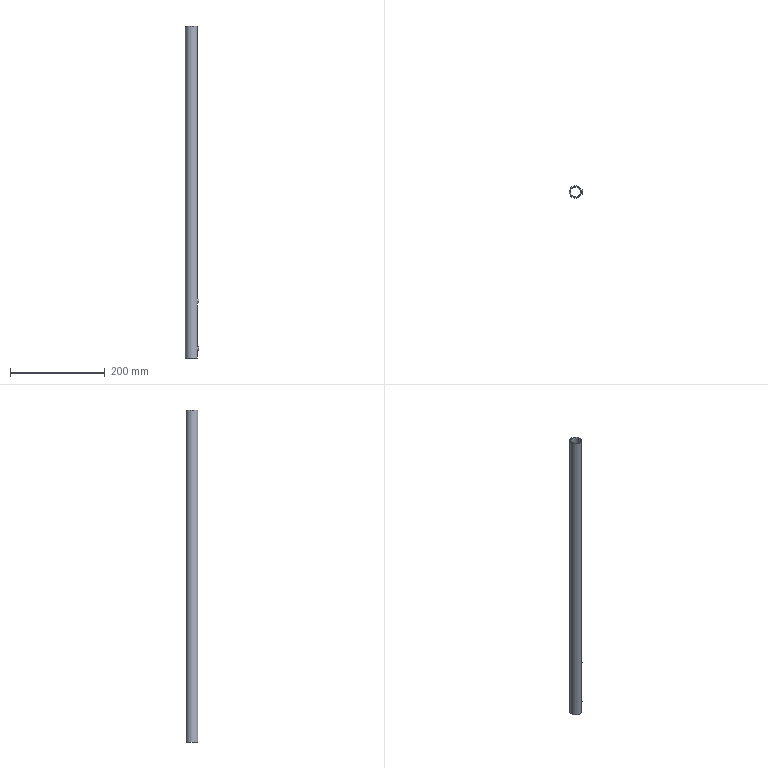Part | STEP file | 1 solid | 24 faces | box 28 x 25 x 700 mm | volume 101372 mm3 | plane 16 | cylinder 4 | cone 4 | commonest cylinder face diameters 4.2 x2 21 x1 25 x1